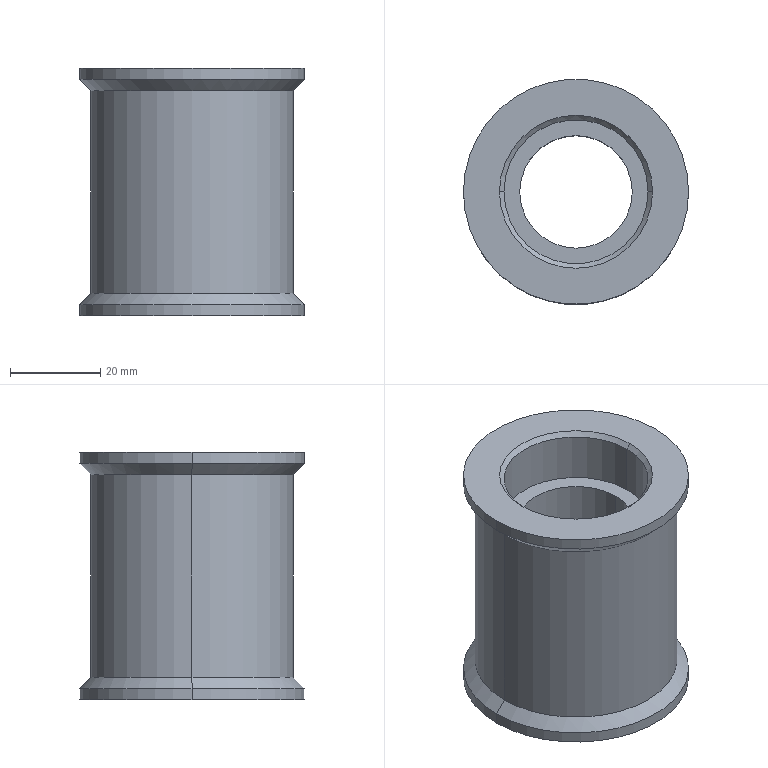Part | SolidWorks | features ICE 3, Chamfer 2, Extrusion 1, MirrorPattern 1 | 1 solid | 24 faces | box 50 x 50 x 55 mm | volume 55634 mm3 | cylinder 12 | cone 8 | plane 4 | commonest cylinder face diameters 32 x4 50 x4 25 x2 45 x2
STEP:
#1=CARTESIAN_POINT('',(22.5,0.,-22.5));
#2=VERTEX_POINT('',#1);
#3=CARTESIAN_POINT('',(-22.5,0.,-22.5));
#4=VERTEX_POINT('',#3);
#5=CARTESIAN_POINT('',(0.,0.,-22.5));
#6=DIRECTION('',(0.,0.,1.));
#7=DIRECTION('',(1.,0.,0.));
#8=AXIS2_PLACEMENT_3D('',#5,#6,#7);
#9=CIRCLE('',#8,22.5);
#10=EDGE_CURVE('',#2,#4,#9,.T.);
#11=ORIENTED_EDGE('',*,*,#10,.F.);
#12=CARTESIAN_POINT('',(25.,0.,-25.));
#13=VERTEX_POINT('',#12);
#14=CARTESIAN_POINT('',(22.5,0.,-22.5));
#15=DIRECTION('',(0.7071,0.,-0.7071));
#16=VECTOR('',#15,1000.);
#17=LINE('',#14,#16);
#18=EDGE_CURVE('',#2,#13,#17,.T.);
#19=ORIENTED_EDGE('',*,*,#18,.T.);
#20=CARTESIAN_POINT('',(-25.,0.,-25.));
#21=VERTEX_POINT('',#20);
#22=CARTESIAN_POINT('',(0.,0.,-25.));
#23=DIRECTION('',(0.,0.,-1.));
#24=DIRECTION('',(1.,0.,0.));
#25=AXIS2_PLACEMENT_3D('',#22,#23,#24);
#26=CIRCLE('',#25,25.);
#27=EDGE_CURVE('',#21,#13,#26,.T.);
#28=ORIENTED_EDGE('',*,*,#27,.F.);
#29=CARTESIAN_POINT('',(-22.5,0.,-22.5));
#30=DIRECTION('',(-0.7071,0.,-0.7071));
#31=VECTOR('',#30,1000.);
#32=LINE('',#29,#31);
#33=EDGE_CURVE('',#4,#21,#32,.T.);
#34=ORIENTED_EDGE('',*,*,#33,.F.);
#35=EDGE_LOOP('',(#11,#19,#28,#34));
#36=FACE_OUTER_BOUND('',#35,.T.);
#37=CARTESIAN_POINT('',(0.,0.,-22.5));
#38=DIRECTION('',(0.,0.,-1.));
#39=DIRECTION('',(-1.,0.,0.));
#40=AXIS2_PLACEMENT_3D('',#37,#38,#39);
#41=CONICAL_SURFACE('',#40,22.5,0.7854);
#42=ADVANCED_FACE('',(#36),#41,.T.);
#43=CARTESIAN_POINT('',(22.5,0.,22.5));
#44=VERTEX_POINT('',#43);
#45=CARTESIAN_POINT('',(-22.5,0.,22.5));
#46=VERTEX_POINT('',#45);
#47=CARTESIAN_POINT('',(0.,0.,22.5));
#48=DIRECTION('',(0.,0.,1.));
#49=DIRECTION('',(1.,0.,0.));
#50=AXIS2_PLACEMENT_3D('',#47,#48,#49);
#51=CIRCLE('',#50,22.5);
#52=EDGE_CURVE('',#44,#46,#51,.T.);
#53=ORIENTED_EDGE('',*,*,#52,.T.);
#54=CARTESIAN_POINT('',(-25.,0.,25.));
#55=VERTEX_POINT('',#54);
#56=CARTESIAN_POINT('',(-25.,0.,25.));
#57=DIRECTION('',(-0.7071,0.,0.7071));
#58=VECTOR('',#57,1000.);
#59=LINE('',#56,#58);
#60=EDGE_CURVE('',#46,#55,#59,.T.);
#61=ORIENTED_EDGE('',*,*,#60,.T.);
#62=CARTESIAN_POINT('',(25.,0.,25.));
#63=VERTEX_POINT('',#62);
#64=CARTESIAN_POINT('',(0.,0.,25.));
#65=DIRECTION('',(0.,0.,1.));
#66=DIRECTION('',(1.,0.,0.));
#67=AXIS2_PLACEMENT_3D('',#64,#65,#66);
#68=CIRCLE('',#67,25.);
#69=EDGE_CURVE('',#63,#55,#68,.T.);
#70=ORIENTED_EDGE('',*,*,#69,.F.);
#71=CARTESIAN_POINT('',(25.,0.,25.));
#72=DIRECTION('',(0.7071,0.,0.7071));
#73=VECTOR('',#72,1000.);
#74=LINE('',#71,#73);
#75=EDGE_CURVE('',#44,#63,#74,.T.);
#76=ORIENTED_EDGE('',*,*,#75,.F.);
#77=EDGE_LOOP('',(#53,#61,#70,#76));
#78=FACE_OUTER_BOUND('',#77,.T.);
#79=CARTESIAN_POINT('',(0.,0.,25.));
#80=DIRECTION('',(0.,0.,1.));
#81=DIRECTION('',(1.,0.,0.));
#82=AXIS2_PLACEMENT_3D('',#79,#80,#81);
#83=CONICAL_SURFACE('',#82,25.,0.7854);
#84=ADVANCED_FACE('',(#78),#83,.T.);
#85=CARTESIAN_POINT('',(-16.,0.,26.5));
#86=VERTEX_POINT('',#85);
#87=CARTESIAN_POINT('',(16.,0.,26.5));
#88=VERTEX_POINT('',#87);
#89=CARTESIAN_POINT('',(0.,0.,26.5));
#90=DIRECTION('',(0.,0.,1.));
#91=DIRECTION('',(1.,0.,0.));
#92=AXIS2_PLACEMENT_3D('',#89,#90,#91);
#93=CIRCLE('',#92,16.);
#94=EDGE_CURVE('',#86,#88,#93,.T.);
#95=ORIENTED_EDGE('',*,*,#94,.F.);
#96=CARTESIAN_POINT('',(-17.,0.,27.5));
#97=VERTEX_POINT('',#96);
#98=CARTESIAN_POINT('',(-17.,0.,27.5));
#99=DIRECTION('',(-0.7071,0.,0.7071));
#100=VECTOR('',#99,1000.);
#101=LINE('',#98,#100);
#102=EDGE_CURVE('',#86,#97,#101,.T.);
#103=ORIENTED_EDGE('',*,*,#102,.T.);
#104=CARTESIAN_POINT('',(17.,0.,27.5));
#105=VERTEX_POINT('',#104);
#106=CARTESIAN_POINT('',(0.,0.,27.5));
#107=DIRECTION('',(0.,0.,-1.));
#108=DIRECTION('',(1.,0.,0.));
#109=AXIS2_PLACEMENT_3D('',#106,#107,#108);
#110=CIRCLE('',#109,17.);
#111=EDGE_CURVE('',#105,#97,#110,.T.);
#112=ORIENTED_EDGE('',*,*,#111,.F.);
#113=CARTESIAN_POINT('',(17.,0.,27.5));
#114=DIRECTION('',(0.7071,0.,0.7071));
#115=VECTOR('',#114,1000.);
#116=LINE('',#113,#115);
#117=EDGE_CURVE('',#88,#105,#116,.T.);
#118=ORIENTED_EDGE('',*,*,#117,.F.);
#119=EDGE_LOOP('',(#95,#103,#112,#118));
#120=FACE_OUTER_BOUND('',#119,.T.);
#121=CARTESIAN_POINT('',(0.,0.,27.5));
#122=DIRECTION('',(0.,0.,1.));
#123=DIRECTION('',(1.,0.,0.));
#124=AXIS2_PLACEMENT_3D('',#121,#122,#123);
#125=CONICAL_SURFACE('',#124,17.,0.7854);
#126=ADVANCED_FACE('',(#120),#125,.F.);
#127=CARTESIAN_POINT('',(16.,0.,-26.5));
#128=VERTEX_POINT('',#127);
#129=CARTESIAN_POINT('',(-16.,0.,-26.5));
#130=VERTEX_POINT('',#129);
#131=CARTESIAN_POINT('',(0.,0.,-26.5));
#132=DIRECTION('',(0.,0.,-1.));
#133=DIRECTION('',(1.,0.,0.));
#134=AXIS2_PLACEMENT_3D('',#131,#132,#133);
#135=CIRCLE('',#134,16.);
#136=EDGE_CURVE('',#128,#130,#135,.T.);
#137=ORIENTED_EDGE('',*,*,#136,.F.);
#138=CARTESIAN_POINT('',(17.,0.,-27.5));
#139=VERTEX_POINT('',#138);
#140=CARTESIAN_POINT('',(16.,0.,-26.5));
#141=DIRECTION('',(0.7071,0.,-0.7071));
#142=VECTOR('',#141,1000.);
#143=LINE('',#140,#142);
#144=EDGE_CURVE('',#128,#139,#143,.T.);
#145=ORIENTED_EDGE('',*,*,#144,.T.);
#146=CARTESIAN_POINT('',(-17.,0.,-27.5));
#147=VERTEX_POINT('',#146);
#148=CARTESIAN_POINT('',(0.,0.,-27.5));
#149=DIRECTION('',(0.,0.,1.));
#150=DIRECTION('',(1.,0.,0.));
#151=AXIS2_PLACEMENT_3D('',#148,#149,#150);
#152=CIRCLE('',#151,17.);
#153=EDGE_CURVE('',#147,#139,#152,.T.);
#154=ORIENTED_EDGE('',*,*,#153,.F.);
#155=CARTESIAN_POINT('',(-16.,0.,-26.5));
#156=DIRECTION('',(-0.7071,0.,-0.7071));
#157=VECTOR('',#156,1000.);
#158=LINE('',#155,#157);
#159=EDGE_CURVE('',#130,#147,#158,.T.);
#160=ORIENTED_EDGE('',*,*,#159,.F.);
#161=EDGE_LOOP('',(#137,#145,#154,#160));
#162=FACE_OUTER_BOUND('',#161,.T.);
#163=CARTESIAN_POINT('',(0.,0.,-26.5));
#164=DIRECTION('',(0.,0.,-1.));
#165=DIRECTION('',(-1.,0.,0.));
#166=AXIS2_PLACEMENT_3D('',#163,#164,#165);
#167=CONICAL_SURFACE('',#166,16.,0.7854);
#168=ADVANCED_FACE('',(#162),#167,.F.);
#169=ORIENTED_EDGE('',*,*,#10,.T.);
#170=CARTESIAN_POINT('',(-22.5,0.,-22.5));
#171=DIRECTION('',(0.,0.,1.));
#172=VECTOR('',#171,1000.);
#173=LINE('',#170,#172);
#174=EDGE_CURVE('',#4,#46,#173,.T.);
#175=ORIENTED_EDGE('',*,*,#174,.T.);
#176=ORIENTED_EDGE('',*,*,#52,.F.);
#177=CARTESIAN_POINT('',(22.5,0.,-22.5));
#178=DIRECTION('',(0.,0.,1.));
#179=VECTOR('',#178,1000.);
#180=LINE('',#177,#179);
#181=EDGE_CURVE('',#2,#44,#180,.T.);
#182=ORIENTED_EDGE('',*,*,#181,.F.);
#183=EDGE_LOOP('',(#169,#175,#176,#182));
#184=FACE_OUTER_BOUND('',#183,.T.);
#185=CARTESIAN_POINT('',(0.,0.,-22.5));
#186=DIRECTION('',(0.,0.,1.));
#187=DIRECTION('',(1.,0.,0.));
#188=AXIS2_PLACEMENT_3D('',#185,#186,#187);
#189=CYLINDRICAL_SURFACE('',#188,22.5);
#190=ADVANCED_FACE('',(#184),#189,.T.);
#191=CARTESIAN_POINT('',(16.,0.,15.5));
#192=VERTEX_POINT('',#191);
#193=CARTESIAN_POINT('',(-16.,0.,15.5));
#194=VERTEX_POINT('',#193);
#195=CARTESIAN_POINT('',(0.,0.,15.5));
#196=DIRECTION('',(0.,0.,-1.));
#197=DIRECTION('',(-1.,0.,0.));
#198=AXIS2_PLACEMENT_3D('',#195,#196,#197);
#199=CIRCLE('',#198,16.);
#200=EDGE_CURVE('',#192,#194,#199,.T.);
#201=ORIENTED_EDGE('',*,*,#200,.T.);
#202=CARTESIAN_POINT('',(-16.,0.,15.5));
#203=DIRECTION('',(0.,0.,1.));
#204=VECTOR('',#203,1000.);
#205=LINE('',#202,#204);
#206=EDGE_CURVE('',#194,#86,#205,.T.);
#207=ORIENTED_EDGE('',*,*,#206,.T.);
#208=ORIENTED_EDGE('',*,*,#94,.T.);
#209=CARTESIAN_POINT('',(16.,0.,15.5));
#210=DIRECTION('',(0.,0.,1.));
#211=VECTOR('',#210,1000.);
#212=LINE('',#209,#211);
#213=EDGE_CURVE('',#192,#88,#212,.T.);
#214=ORIENTED_EDGE('',*,*,#213,.F.);
#215=EDGE_LOOP('',(#201,#207,#208,#214));
#216=FACE_OUTER_BOUND('',#215,.T.);
#217=CARTESIAN_POINT('',(0.,0.,15.5));
#218=DIRECTION('',(0.,0.,1.));
#219=DIRECTION('',(1.,0.,0.));
#220=AXIS2_PLACEMENT_3D('',#217,#218,#219);
#221=CYLINDRICAL_SURFACE('',#220,16.);
#222=ADVANCED_FACE('',(#216),#221,.F.);
#223=CARTESIAN_POINT('',(16.,0.,-15.5));
#224=VERTEX_POINT('',#223);
#225=CARTESIAN_POINT('',(-16.,0.,-15.5));
#226=VERTEX_POINT('',#225);
#227=CARTESIAN_POINT('',(0.,0.,-15.5));
#228=DIRECTION('',(0.,0.,-1.));
#229=DIRECTION('',(-1.,0.,0.));
#230=AXIS2_PLACEMENT_3D('',#227,#228,#229);
#231=CIRCLE('',#230,16.);
#232=EDGE_CURVE('',#224,#226,#231,.T.);
#233=ORIENTED_EDGE('',*,*,#232,.F.);
#234=CARTESIAN_POINT('',(16.,0.,-15.5));
#235=DIRECTION('',(0.,0.,-1.));
#236=VECTOR('',#235,1000.);
#237=LINE('',#234,#236);
#238=EDGE_CURVE('',#224,#128,#237,.T.);
#239=ORIENTED_EDGE('',*,*,#238,.T.);
#240=ORIENTED_EDGE('',*,*,#136,.T.);
#241=CARTESIAN_POINT('',(-16.,0.,-15.5));
#242=DIRECTION('',(0.,0.,-1.));
#243=VECTOR('',#242,1000.);
#244=LINE('',#241,#243);
#245=EDGE_CURVE('',#226,#130,#244,.T.);
#246=ORIENTED_EDGE('',*,*,#245,.F.);
#247=EDGE_LOOP('',(#233,#239,#240,#246));
#248=FACE_OUTER_BOUND('',#247,.T.);
#249=CARTESIAN_POINT('',(0.,0.,-15.5));
#250=DIRECTION('',(0.,0.,-1.));
#251=DIRECTION('',(-1.,0.,0.));
#252=AXIS2_PLACEMENT_3D('',#249,#250,#251);
#253=CYLINDRICAL_SURFACE('',#252,16.);
#254=ADVANCED_FACE('',(#248),#253,.F.);
#255=CARTESIAN_POINT('',(25.,0.,27.5));
#256=VERTEX_POINT('',#255);
#257=CARTESIAN_POINT('',(-25.,0.,27.5));
#258=VERTEX_POINT('',#257);
#259=CARTESIAN_POINT('',(0.,0.,27.5));
#260=DIRECTION('',(0.,0.,1.));
#261=DIRECTION('',(1.,0.,0.));
#262=AXIS2_PLACEMENT_3D('',#259,#260,#261);
#263=CIRCLE('',#262,25.);
#264=EDGE_CURVE('',#256,#258,#263,.T.);
#265=ORIENTED_EDGE('',*,*,#264,.F.);
#266=CARTESIAN_POINT('',(25.,0.,27.5));
#267=DIRECTION('',(0.,0.,-1.));
#268=VECTOR('',#267,1000.);
#269=LINE('',#266,#268);
#270=EDGE_CURVE('',#256,#63,#269,.T.);
#271=ORIENTED_EDGE('',*,*,#270,.T.);
#272=ORIENTED_EDGE('',*,*,#69,.T.);
#273=CARTESIAN_POINT('',(-25.,0.,27.5));
#274=DIRECTION('',(0.,0.,-1.));
#275=VECTOR('',#274,1000.);
#276=LINE('',#273,#275);
#277=EDGE_CURVE('',#258,#55,#276,.T.);
#278=ORIENTED_EDGE('',*,*,#277,.F.);
#279=EDGE_LOOP('',(#265,#271,#272,#278));
#280=FACE_OUTER_BOUND('',#279,.T.);
#281=CARTESIAN_POINT('',(0.,0.,27.5));
#282=DIRECTION('',(0.,0.,-1.));
#283=DIRECTION('',(-1.,0.,0.));
#284=AXIS2_PLACEMENT_3D('',#281,#282,#283);
#285=CYLINDRICAL_SURFACE('',#284,25.);
#286=ADVANCED_FACE('',(#280),#285,.T.);
#287=CARTESIAN_POINT('',(12.5,0.,15.5));
#288=VERTEX_POINT('',#287);
#289=CARTESIAN_POINT('',(-12.5,0.,15.5));
#290=VERTEX_POINT('',#289);
#291=CARTESIAN_POINT('',(0.,0.,15.5));
#292=DIRECTION('',(0.,0.,-1.));
#293=DIRECTION('',(1.,0.,0.));
#294=AXIS2_PLACEMENT_3D('',#291,#292,#293);
#295=CIRCLE('',#294,12.5);
#296=EDGE_CURVE('',#288,#290,#295,.T.);
#297=ORIENTED_EDGE('',*,*,#296,.F.);
#298=CARTESIAN_POINT('',(12.5,0.,-15.5));
#299=VERTEX_POINT('',#298);
#300=CARTESIAN_POINT('',(12.5,0.,27.5));
#301=DIRECTION('',(0.,0.,-1.));
#302=VECTOR('',#301,1000.);
#303=LINE('',#300,#302);
#304=EDGE_CURVE('',#288,#299,#303,.T.);
#305=ORIENTED_EDGE('',*,*,#304,.T.);
#306=CARTESIAN_POINT('',(-12.5,0.,-15.5));
#307=VERTEX_POINT('',#306);
#308=CARTESIAN_POINT('',(0.,0.,-15.5));
#309=DIRECTION('',(0.,0.,1.));
#310=DIRECTION('',(-1.,0.,0.));
#311=AXIS2_PLACEMENT_3D('',#308,#309,#310);
#312=CIRCLE('',#311,12.5);
#313=EDGE_CURVE('',#307,#299,#312,.T.);
#314=ORIENTED_EDGE('',*,*,#313,.F.);
#315=CARTESIAN_POINT('',(-12.5,0.,27.5));
#316=DIRECTION('',(0.,0.,-1.));
#317=VECTOR('',#316,1000.);
#318=LINE('',#315,#317);
#319=EDGE_CURVE('',#290,#307,#318,.T.);
#320=ORIENTED_EDGE('',*,*,#319,.F.);
#321=EDGE_LOOP('',(#297,#305,#314,#320));
#322=FACE_OUTER_BOUND('',#321,.T.);
#323=CARTESIAN_POINT('',(0.,0.,27.5));
#324=DIRECTION('',(0.,0.,-1.));
#325=DIRECTION('',(-1.,0.,0.));
#326=AXIS2_PLACEMENT_3D('',#323,#324,#325);
#327=CYLINDRICAL_SURFACE('',#326,12.5);
#328=ADVANCED_FACE('',(#322),#327,.F.);
#329=ORIENTED_EDGE('',*,*,#27,.T.);
#330=CARTESIAN_POINT('',(25.,0.,-27.5));
#331=VERTEX_POINT('',#330);
#332=CARTESIAN_POINT('',(25.,0.,27.5));
#333=DIRECTION('',(0.,0.,-1.));
#334=VECTOR('',#333,1000.);
#335=LINE('',#332,#334);
#336=EDGE_CURVE('',#13,#331,#335,.T.);
#337=ORIENTED_EDGE('',*,*,#336,.T.);
#338=CARTESIAN_POINT('',(-25.,0.,-27.5));
#339=VERTEX_POINT('',#338);
#340=CARTESIAN_POINT('',(0.,0.,-27.5));
#341=DIRECTION('',(0.,0.,1.));
#342=DIRECTION('',(1.,0.,0.));
#343=AXIS2_PLACEMENT_3D('',#340,#341,#342);
#344=CIRCLE('',#343,25.);
#345=EDGE_CURVE('',#331,#339,#344,.T.);
#346=ORIENTED_EDGE('',*,*,#345,.T.);
#347=CARTESIAN_POINT('',(-25.,0.,27.5));
#348=DIRECTION('',(0.,0.,-1.));
#349=VECTOR('',#348,1000.);
#350=LINE('',#347,#349);
#351=EDGE_CURVE('',#21,#339,#350,.T.);
#352=ORIENTED_EDGE('',*,*,#351,.F.);
#353=EDGE_LOOP('',(#329,#337,#346,#352));
#354=FACE_OUTER_BOUND('',#353,.T.);
#355=CARTESIAN_POINT('',(0.,0.,27.5));
#356=DIRECTION('',(0.,0.,-1.));
#357=DIRECTION('',(-1.,0.,0.));
#358=AXIS2_PLACEMENT_3D('',#355,#356,#357);
#359=CYLINDRICAL_SURFACE('',#358,25.);
#360=ADVANCED_FACE('',(#354),#359,.T.);
#361=ORIENTED_EDGE('',*,*,#336,.F.);
#362=CARTESIAN_POINT('',(0.,0.,-25.));
#363=DIRECTION('',(0.,0.,-1.));
#364=DIRECTION('',(1.,0.,0.));
#365=AXIS2_PLACEMENT_3D('',#362,#363,#364);
#366=CIRCLE('',#365,25.);
#367=EDGE_CURVE('',#13,#21,#366,.T.);
#368=ORIENTED_EDGE('',*,*,#367,.T.);
#369=ORIENTED_EDGE('',*,*,#351,.T.);
#370=CARTESIAN_POINT('',(0.,0.,-27.5));
#371=DIRECTION('',(0.,0.,1.));
#372=DIRECTION('',(1.,0.,0.));
#373=AXIS2_PLACEMENT_3D('',#370,#371,#372);
#374=CIRCLE('',#373,25.);
#375=EDGE_CURVE('',#339,#331,#374,.T.);
#376=ORIENTED_EDGE('',*,*,#375,.T.);
#377=EDGE_LOOP('',(#361,#368,#369,#376));
#378=FACE_OUTER_BOUND('',#377,.T.);
#379=CARTESIAN_POINT('',(0.,0.,27.5));
#380=DIRECTION('',(0.,0.,-1.));
#381=DIRECTION('',(-1.,0.,0.));
#382=AXIS2_PLACEMENT_3D('',#379,#380,#381);
#383=CYLINDRICAL_SURFACE('',#382,25.);
#384=ADVANCED_FACE('',(#378),#383,.T.);
#385=ORIENTED_EDGE('',*,*,#304,.F.);
#386=CARTESIAN_POINT('',(0.,0.,15.5));
#387=DIRECTION('',(0.,0.,-1.));
#388=DIRECTION('',(1.,0.,0.));
#389=AXIS2_PLACEMENT_3D('',#386,#387,#388);
#390=CIRCLE('',#389,12.5);
#391=EDGE_CURVE('',#290,#288,#390,.T.);
#392=ORIENTED_EDGE('',*,*,#391,.F.);
#393=ORIENTED_EDGE('',*,*,#319,.T.);
#394=CARTESIAN_POINT('',(0.,0.,-15.5));
#395=DIRECTION('',(0.,0.,1.));
#396=DIRECTION('',(-1.,0.,0.));
#397=AXIS2_PLACEMENT_3D('',#394,#395,#396);
#398=CIRCLE('',#397,12.5);
#399=EDGE_CURVE('',#299,#307,#398,.T.);
#400=ORIENTED_EDGE('',*,*,#399,.F.);
#401=EDGE_LOOP('',(#385,#392,#393,#400));
#402=FACE_OUTER_BOUND('',#401,.T.);
#403=CARTESIAN_POINT('',(0.,0.,27.5));
#404=DIRECTION('',(0.,0.,-1.));
#405=DIRECTION('',(-1.,0.,0.));
#406=AXIS2_PLACEMENT_3D('',#403,#404,#405);
#407=CYLINDRICAL_SURFACE('',#406,12.5);
#408=ADVANCED_FACE('',(#402),#407,.F.);
#409=ORIENTED_EDGE('',*,*,#270,.F.);
#410=CARTESIAN_POINT('',(0.,0.,27.5));
#411=DIRECTION('',(0.,0.,1.));
#412=DIRECTION('',(1.,0.,0.));
#413=AXIS2_PLACEMENT_3D('',#410,#411,#412);
#414=CIRCLE('',#413,25.);
#415=EDGE_CURVE('',#258,#256,#414,.T.);
#416=ORIENTED_EDGE('',*,*,#415,.F.);
#417=ORIENTED_EDGE('',*,*,#277,.T.);
#418=CARTESIAN_POINT('',(0.,0.,25.));
#419=DIRECTION('',(0.,0.,1.));
#420=DIRECTION('',(1.,0.,0.));
#421=AXIS2_PLACEMENT_3D('',#418,#419,#420);
#422=CIRCLE('',#421,25.);
#423=EDGE_CURVE('',#55,#63,#422,.T.);
#424=ORIENTED_EDGE('',*,*,#423,.T.);
#425=EDGE_LOOP('',(#409,#416,#417,#424));
#426=FACE_OUTER_BOUND('',#425,.T.);
#427=CARTESIAN_POINT('',(0.,0.,27.5));
#428=DIRECTION('',(0.,0.,-1.));
#429=DIRECTION('',(-1.,0.,0.));
#430=AXIS2_PLACEMENT_3D('',#427,#428,#429);
#431=CYLINDRICAL_SURFACE('',#430,25.);
#432=ADVANCED_FACE('',(#426),#431,.T.);
#433=ORIENTED_EDGE('',*,*,#111,.T.);
#434=CARTESIAN_POINT('',(0.,0.,27.5));
#435=DIRECTION('',(0.,0.,-1.));
#436=DIRECTION('',(1.,0.,0.));
#437=AXIS2_PLACEMENT_3D('',#434,#435,#436);
#438=CIRCLE('',#437,17.);
#439=EDGE_CURVE('',#97,#105,#438,.T.);
#440=ORIENTED_EDGE('',*,*,#439,.T.);
#441=EDGE_LOOP('',(#433,#440));
#442=FACE_BOUND('',#441,.T.);
#443=ORIENTED_EDGE('',*,*,#415,.T.);
#444=ORIENTED_EDGE('',*,*,#264,.T.);
#445=EDGE_LOOP('',(#443,#444));
#446=FACE_OUTER_BOUND('',#445,.T.);
#447=CARTESIAN_POINT('',(0.,0.,27.5));
#448=DIRECTION('',(0.,0.,1.));
#449=DIRECTION('',(1.,0.,0.));
#450=AXIS2_PLACEMENT_3D('',#447,#448,#449);
#451=PLANE('',#450);
#452=ADVANCED_FACE('',(#442,#446),#451,.T.);
#453=ORIENTED_EDGE('',*,*,#153,.T.);
#454=CARTESIAN_POINT('',(0.,0.,-27.5));
#455=DIRECTION('',(0.,0.,1.));
#456=DIRECTION('',(1.,0.,0.));
#457=AXIS2_PLACEMENT_3D('',#454,#455,#456);
#458=CIRCLE('',#457,17.);
#459=EDGE_CURVE('',#139,#147,#458,.T.);
#460=ORIENTED_EDGE('',*,*,#459,.T.);
#461=EDGE_LOOP('',(#453,#460));
#462=FACE_BOUND('',#461,.T.);
#463=ORIENTED_EDGE('',*,*,#375,.F.);
#464=ORIENTED_EDGE('',*,*,#345,.F.);
#465=EDGE_LOOP('',(#463,#464));
#466=FACE_OUTER_BOUND('',#465,.T.);
#467=CARTESIAN_POINT('',(0.,0.,-27.5));
#468=DIRECTION('',(0.,0.,1.));
#469=DIRECTION('',(1.,0.,0.));
#470=AXIS2_PLACEMENT_3D('',#467,#468,#469);
#471=PLANE('',#470);
#472=ADVANCED_FACE('',(#462,#466),#471,.F.);
#473=CARTESIAN_POINT('',(0.,0.,-15.5));
#474=DIRECTION('',(0.,0.,-1.));
#475=DIRECTION('',(-1.,0.,0.));
#476=AXIS2_PLACEMENT_3D('',#473,#474,#475);
#477=CIRCLE('',#476,16.);
#478=EDGE_CURVE('',#226,#224,#477,.T.);
#479=ORIENTED_EDGE('',*,*,#478,.T.);
#480=ORIENTED_EDGE('',*,*,#232,.T.);
#481=EDGE_LOOP('',(#479,#480));
#482=FACE_OUTER_BOUND('',#481,.T.);
#483=ORIENTED_EDGE('',*,*,#313,.T.);
#484=ORIENTED_EDGE('',*,*,#399,.T.);
#485=EDGE_LOOP('',(#483,#484));
#486=FACE_BOUND('',#485,.T.);
#487=CARTESIAN_POINT('',(0.,0.,-15.5));
#488=DIRECTION('',(0.,0.,-1.));
#489=DIRECTION('',(-1.,0.,0.));
#490=AXIS2_PLACEMENT_3D('',#487,#488,#489);
#491=PLANE('',#490);
#492=ADVANCED_FACE('',(#482,#486),#491,.T.);
#493=ORIENTED_EDGE('',*,*,#238,.F.);
#494=ORIENTED_EDGE('',*,*,#478,.F.);
#495=ORIENTED_EDGE('',*,*,#245,.T.);
#496=CARTESIAN_POINT('',(0.,0.,-26.5));
#497=DIRECTION('',(0.,0.,-1.));
#498=DIRECTION('',(1.,0.,0.));
#499=AXIS2_PLACEMENT_3D('',#496,#497,#498);
#500=CIRCLE('',#499,16.);
#501=EDGE_CURVE('',#130,#128,#500,.T.);
#502=ORIENTED_EDGE('',*,*,#501,.T.);
#503=EDGE_LOOP('',(#493,#494,#495,#502));
#504=FACE_OUTER_BOUND('',#503,.T.);
#505=CARTESIAN_POINT('',(0.,0.,-15.5));
#506=DIRECTION('',(0.,0.,-1.));
#507=DIRECTION('',(-1.,0.,0.));
#508=AXIS2_PLACEMENT_3D('',#505,#506,#507);
#509=CYLINDRICAL_SURFACE('',#508,16.);
#510=ADVANCED_FACE('',(#504),#509,.F.);
#511=ORIENTED_EDGE('',*,*,#200,.F.);
#512=CARTESIAN_POINT('',(0.,0.,15.5));
#513=DIRECTION('',(0.,0.,-1.));
#514=DIRECTION('',(-1.,0.,0.));
#515=AXIS2_PLACEMENT_3D('',#512,#513,#514);
#516=CIRCLE('',#515,16.);
#517=EDGE_CURVE('',#194,#192,#516,.T.);
#518=ORIENTED_EDGE('',*,*,#517,.F.);
#519=EDGE_LOOP('',(#511,#518));
#520=FACE_OUTER_BOUND('',#519,.T.);
#521=ORIENTED_EDGE('',*,*,#391,.T.);
#522=ORIENTED_EDGE('',*,*,#296,.T.);
#523=EDGE_LOOP('',(#521,#522));
#524=FACE_BOUND('',#523,.T.);
#525=CARTESIAN_POINT('',(0.,0.,15.5));
#526=DIRECTION('',(0.,0.,1.));
#527=DIRECTION('',(-1.,0.,0.));
#528=AXIS2_PLACEMENT_3D('',#525,#526,#527);
#529=PLANE('',#528);
#530=ADVANCED_FACE('',(#520,#524),#529,.T.);
#531=ORIENTED_EDGE('',*,*,#206,.F.);
#532=ORIENTED_EDGE('',*,*,#517,.T.);
#533=ORIENTED_EDGE('',*,*,#213,.T.);
#534=CARTESIAN_POINT('',(0.,0.,26.5));
#535=DIRECTION('',(0.,0.,1.));
#536=DIRECTION('',(1.,0.,0.));
#537=AXIS2_PLACEMENT_3D('',#534,#535,#536);
#538=CIRCLE('',#537,16.);
#539=EDGE_CURVE('',#88,#86,#538,.T.);
#540=ORIENTED_EDGE('',*,*,#539,.T.);
#541=EDGE_LOOP('',(#531,#532,#533,#540));
#542=FACE_OUTER_BOUND('',#541,.T.);
#543=CARTESIAN_POINT('',(0.,0.,15.5));
#544=DIRECTION('',(0.,0.,1.));
#545=DIRECTION('',(1.,0.,0.));
#546=AXIS2_PLACEMENT_3D('',#543,#544,#545);
#547=CYLINDRICAL_SURFACE('',#546,16.);
#548=ADVANCED_FACE('',(#542),#547,.F.);
#549=ORIENTED_EDGE('',*,*,#174,.F.);
#550=CARTESIAN_POINT('',(0.,0.,-22.5));
#551=DIRECTION('',(0.,0.,1.));
#552=DIRECTION('',(1.,0.,0.));
#553=AXIS2_PLACEMENT_3D('',#550,#551,#552);
#554=CIRCLE('',#553,22.5);
#555=EDGE_CURVE('',#4,#2,#554,.T.);
#556=ORIENTED_EDGE('',*,*,#555,.T.);
#557=ORIENTED_EDGE('',*,*,#181,.T.);
#558=CARTESIAN_POINT('',(0.,0.,22.5));
#559=DIRECTION('',(0.,0.,1.));
#560=DIRECTION('',(1.,0.,0.));
#561=AXIS2_PLACEMENT_3D('',#558,#559,#560);
#562=CIRCLE('',#561,22.5);
#563=EDGE_CURVE('',#46,#44,#562,.T.);
#564=ORIENTED_EDGE('',*,*,#563,.F.);
#565=EDGE_LOOP('',(#549,#556,#557,#564));
#566=FACE_OUTER_BOUND('',#565,.T.);
#567=CARTESIAN_POINT('',(0.,0.,-22.5));
#568=DIRECTION('',(0.,0.,1.));
#569=DIRECTION('',(1.,0.,0.));
#570=AXIS2_PLACEMENT_3D('',#567,#568,#569);
#571=CYLINDRICAL_SURFACE('',#570,22.5);
#572=ADVANCED_FACE('',(#566),#571,.T.);
#573=ORIENTED_EDGE('',*,*,#144,.F.);
#574=ORIENTED_EDGE('',*,*,#501,.F.);
#575=ORIENTED_EDGE('',*,*,#159,.T.);
#576=ORIENTED_EDGE('',*,*,#459,.F.);
#577=EDGE_LOOP('',(#573,#574,#575,#576));
#578=FACE_OUTER_BOUND('',#577,.T.);
#579=CARTESIAN_POINT('',(0.,0.,-26.5));
#580=DIRECTION('',(0.,0.,-1.));
#581=DIRECTION('',(-1.,0.,0.));
#582=AXIS2_PLACEMENT_3D('',#579,#580,#581);
#583=CONICAL_SURFACE('',#582,16.,0.7854);
#584=ADVANCED_FACE('',(#578),#583,.F.);
#585=ORIENTED_EDGE('',*,*,#102,.F.);
#586=ORIENTED_EDGE('',*,*,#539,.F.);
#587=ORIENTED_EDGE('',*,*,#117,.T.);
#588=ORIENTED_EDGE('',*,*,#439,.F.);
#589=EDGE_LOOP('',(#585,#586,#587,#588));
#590=FACE_OUTER_BOUND('',#589,.T.);
#591=CARTESIAN_POINT('',(0.,0.,27.5));
#592=DIRECTION('',(0.,0.,1.));
#593=DIRECTION('',(1.,0.,0.));
#594=AXIS2_PLACEMENT_3D('',#591,#592,#593);
#595=CONICAL_SURFACE('',#594,17.,0.7854);
#596=ADVANCED_FACE('',(#590),#595,.F.);
#597=ORIENTED_EDGE('',*,*,#60,.F.);
#598=ORIENTED_EDGE('',*,*,#563,.T.);
#599=ORIENTED_EDGE('',*,*,#75,.T.);
#600=ORIENTED_EDGE('',*,*,#423,.F.);
#601=EDGE_LOOP('',(#597,#598,#599,#600));
#602=FACE_OUTER_BOUND('',#601,.T.);
#603=CARTESIAN_POINT('',(0.,0.,25.));
#604=DIRECTION('',(0.,0.,1.));
#605=DIRECTION('',(1.,0.,0.));
#606=AXIS2_PLACEMENT_3D('',#603,#604,#605);
#607=CONICAL_SURFACE('',#606,25.,0.7854);
#608=ADVANCED_FACE('',(#602),#607,.T.);
#609=ORIENTED_EDGE('',*,*,#18,.F.);
#610=ORIENTED_EDGE('',*,*,#555,.F.);
#611=ORIENTED_EDGE('',*,*,#33,.T.);
#612=ORIENTED_EDGE('',*,*,#367,.F.);
#613=EDGE_LOOP('',(#609,#610,#611,#612));
#614=FACE_OUTER_BOUND('',#613,.T.);
#615=CARTESIAN_POINT('',(0.,0.,-22.5));
#616=DIRECTION('',(0.,0.,-1.));
#617=DIRECTION('',(-1.,0.,0.));
#618=AXIS2_PLACEMENT_3D('',#615,#616,#617);
#619=CONICAL_SURFACE('',#618,22.5,0.7854);
#620=ADVANCED_FACE('',(#614),#619,.T.);
#621=CLOSED_SHELL('',(#42,#84,#126,#168,#190,#222,#254,#286,#328,#360,#384,#408,#432,#452,#472,#492,#510,#530,#548,#572,#584,#596,#608,#620));
#622=MANIFOLD_SOLID_BREP('',#621);
#623=CARTESIAN_POINT('',(0.,0.,0.));
#624=DIRECTION('',(0.,0.,1.));
#625=DIRECTION('',(1.,0.,0.));
#626=AXIS2_PLACEMENT_3D('',#623,#624,#625);
#627=(LENGTH_UNIT()NAMED_UNIT(*)SI_UNIT(.MILLI.,.METRE.));
#628=UNCERTAINTY_MEASURE_WITH_UNIT(LENGTH_MEASURE(0.00001),#627,'','');
#629=(NAMED_UNIT(*)PLANE_ANGLE_UNIT()SI_UNIT($,.RADIAN.));
#630=(NAMED_UNIT(*)SI_UNIT($,.STERADIAN.)SOLID_ANGLE_UNIT());
#631=(GEOMETRIC_REPRESENTATION_CONTEXT(3)GLOBAL_UNCERTAINTY_ASSIGNED_CONTEXT((#628))GLOBAL_UNIT_ASSIGNED_CONTEXT((#627,#629,#630))REPRESENTATION_CONTEXT('',''));
#632=ADVANCED_BREP_SHAPE_REPRESENTATION('',(#622,#626),#631);